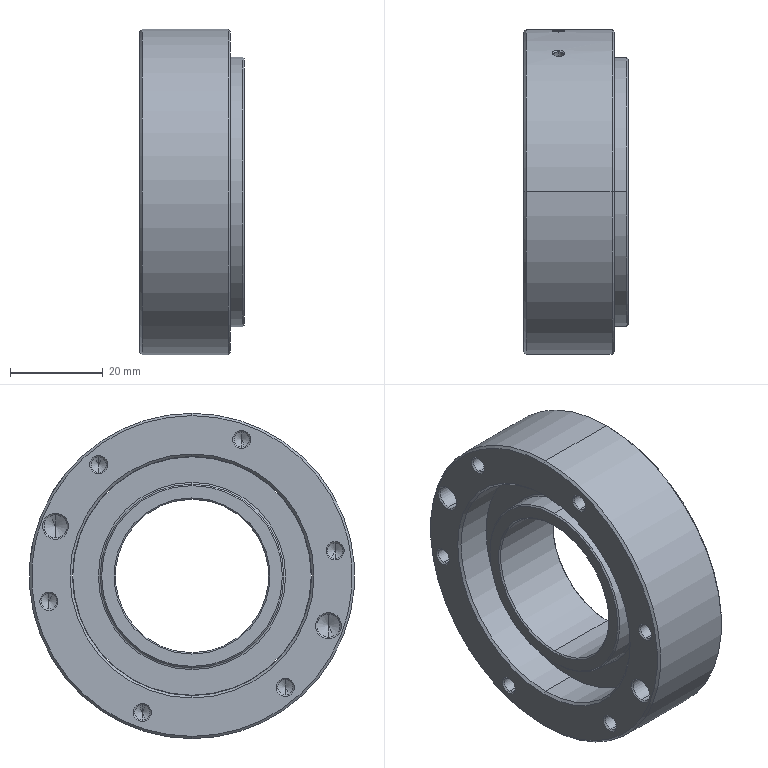Part | SolidWorks | features BaseBody 2 | 2 solids | 165 faces | box 22.5 x 70 x 70 mm | volume 47799 mm3 | cone 90 | cylinder 56 | plane 11 | torus 4 | spline 4 | commonest cylinder face diameters 2.5 x14 3.3 x12 2.1 x4 5 x4 51.3 x4 51.5 x4